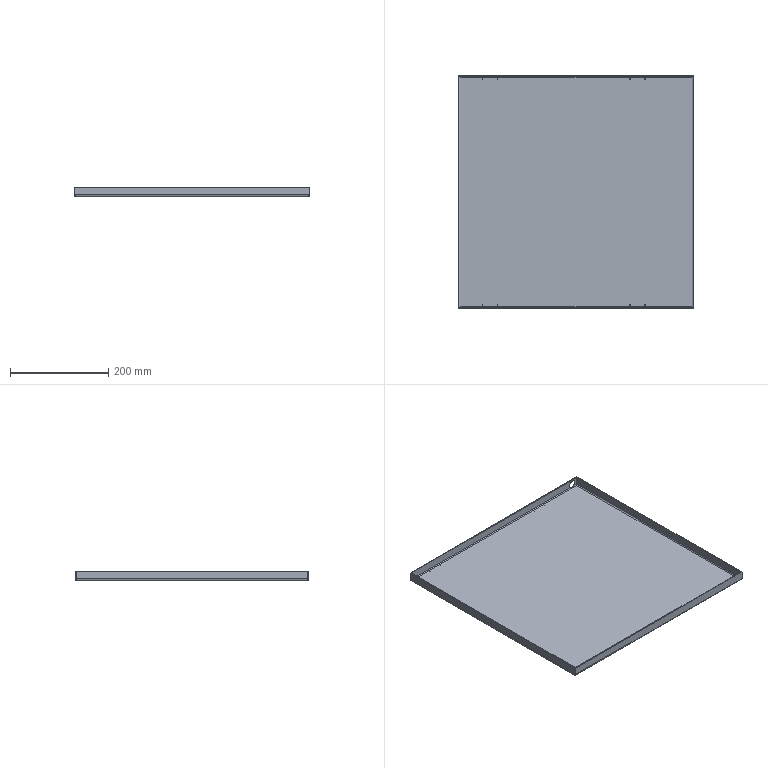Part | NX | features solid 2 | 1 solid | 65 faces | box 480 x 475 x 20 mm | volume 519123 mm3 | plane 38 | cylinder 26 | spline 1 | commonest cylinder face diameters 1 x16 4 x4 8 x4 15 x2